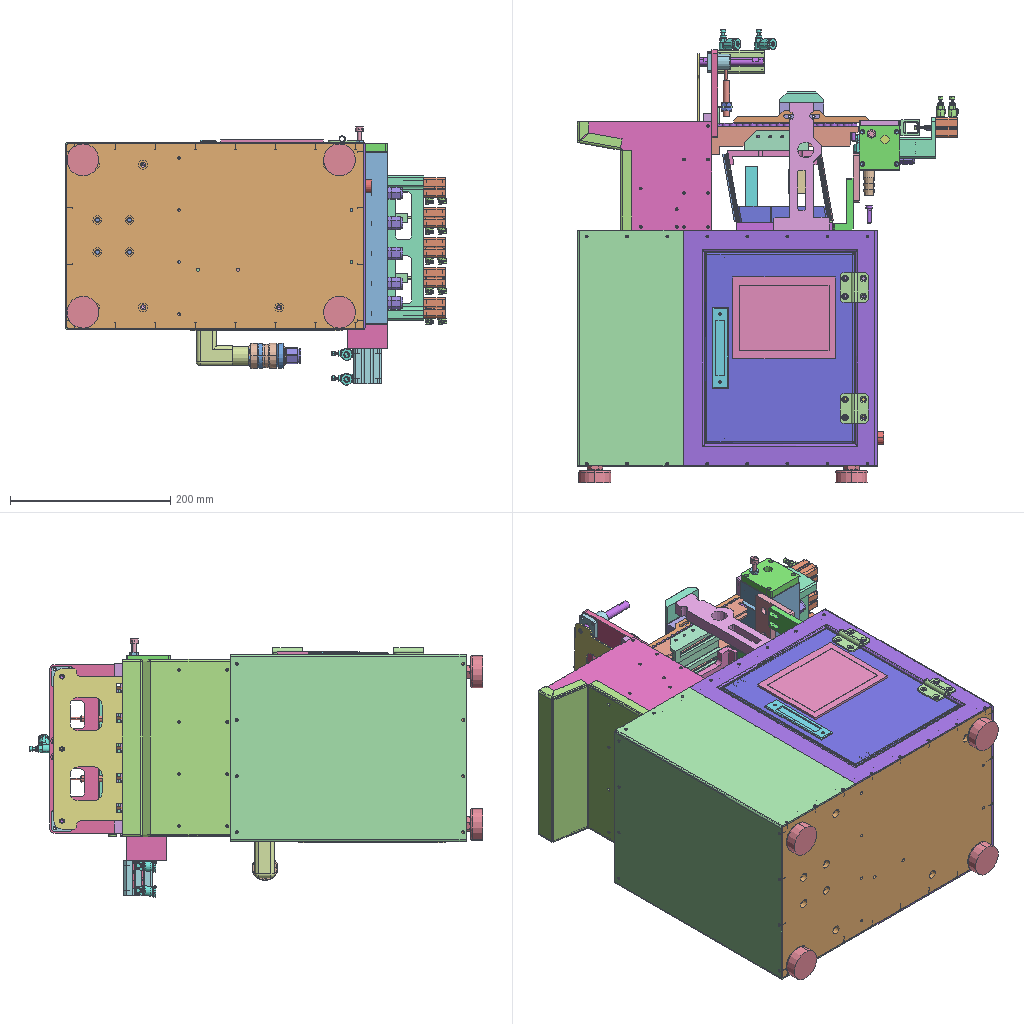Assembly | STEP file | 103 different items | 523 placed | box 476 x 566 x 322 mm
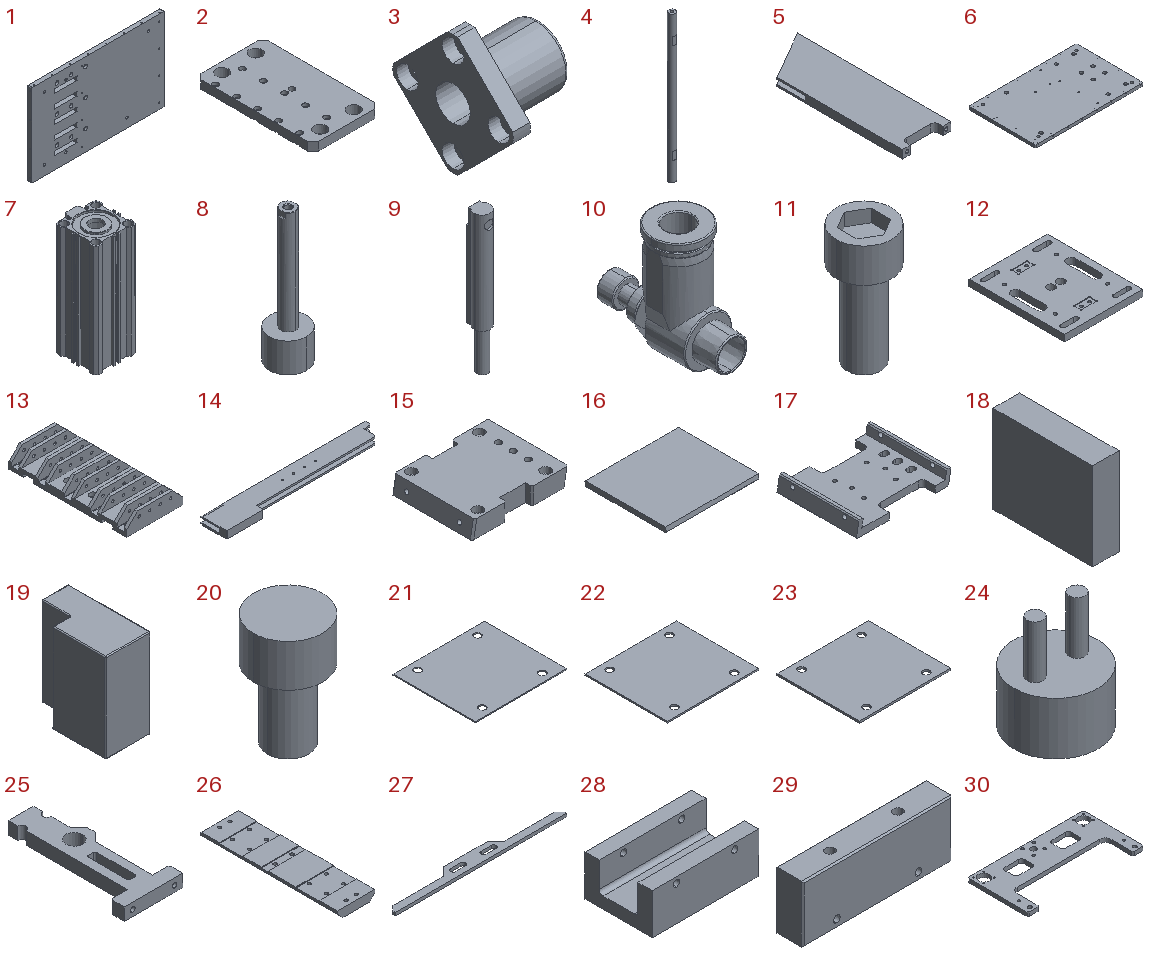Parts list (item | name | quantity | parent item | size | volume):
1 | GLSJ-10-27_default | x1 | in 202 | 370 x 12 x 230 mm | 950756 mm3
2 | GLSJ-10-31_default | x1 | in Lifting mechanism_default | 120 x 210 x 15 mm | 339737 mm3
3 | LBHSW12_default | x4 | in Lifting mechanism_default | 30 x 42 x 42 mm | 10118 mm3
4 | GLSJ-10-30_default | x6 | in Lifting mechanism_default | 12 x 12 x 272 mm | 29884 mm3
5 | GLSJ-10-32_default | x5 | in Lifting mechanism_default | 60 x 188.591 x 10 mm | 87112 mm3
6 | GLSJ-10-28_default | x1 | in Lifting mechanism_default | 370 x 230 x 10 mm | 831396 mm3
7 | HI_JSNR40X100_body_default | x1 | in JSNR40X100TD-2_07_-tab_default | 52 x 57 x 139.5 mm | 157789 mm3
8 | HI_JSNR40X100_rod_default | x1 | in JSNR40X100TD-2_07_-tab_default | 40 x 40 x 142.5 mm | 61393 mm3
9 | HI_TD-11-jsn_default | x6 | in JSNR40X100TD-2_07_-tab_default, JSNR16X30TD-2_02_-tab_default, JSNR20X15TD-2_03_-tab_default | 4 x 4.5 x 35.5 mm | 415.649 mm3
10 | KZB668-08-01-668 | x2 | in JSNR40X100TD-2_07_-tab_default | 16 x 36.5 x 33.35 mm | 5183 mm3
11 | M8 screw | x1 | in Lifting mechanism_default | 13 x 13 x 28 mm | 1901 mm3
12 | GLSJ-10-48_default | x1 | in Vibrator section_default | 120 x 147 x 10 mm | 151449 mm3
13 | GLSJ-10-12_default | x1 | in Vibrator section_default | 80 x 168 x 25 mm | 122709 mm3
14 | GLSJ-10-11_default | x5 | in Vibrator section_default | 223 x 35 x 10 mm | 29153 mm3
15 | GLSJ-10-44_default | x1 | in Vibrator_default | 113.527 x 95 x 20 mm | 189360 mm3
16 | Vibrator side plate_default | x2 | in Vibrator_default | 95 x 83.558 x 5 mm | 39344 mm3
17 | GLSJ-10-42_default | x1 | in Vibrator_default | 112.85 x 95 x 18 mm | 76999 mm3
18 | Vibrator coil left support_default | x1 | in Vibrator_default | 15 x 57 x 50 mm | 41837 mm3
19 | GLSJ-10-43_default | x1 | in Vibrator_default | 25 x 46 x 50 mm | 48561 mm3
20 | m6-15 | x5 | in Vibrator_default | 10 x 10 x 16.1 mm | 761.836 mm3
21 | GLSJ-10-45 | x10 | in Leaf spring assembly | 95 x 85 x 1 mm | 7921 mm3
22 | GLSJ-10-46 | x1 | in Vibrator_default | 95 x 85 x 1.5 mm | 11882 mm3
23 | GLSJ-10-47 | x1 | in Vibrator_default | 95 x 85 x 2 mm | 15842 mm3
24 | 332 | x1 | in Vibrator section_default | 8 x 8 x 10.1 mm | 269.13 mm3
25 | GLSJ-10-13_default | x2 | in Pressing mechanism_default | 70 x 159 x 15 mm | 69030 mm3
26 | GLSJ-10-14_default | x1 | in Pressing mechanism_default | 55 x 200 x 14 mm | 124098 mm3
27 | GLSJ-10-17_default | x5 | in Pressing mechanism_default | 170 x 15 x 3 mm | 4325 mm3
28 | GLSJ-10-15_default | x2 | in Pressing mechanism_default | 55 x 34.5 x 21 mm | 22837 mm3
29 | GLSJ-10-16_default | x1 | in Pressing mechanism_default | 55 x 10 x 21 mm | 11236 mm3
30 | GLSJ-10-21_default | x1 | in Scraper mechanism_default | 210 x 110 x 7 mm | 83543 mm3
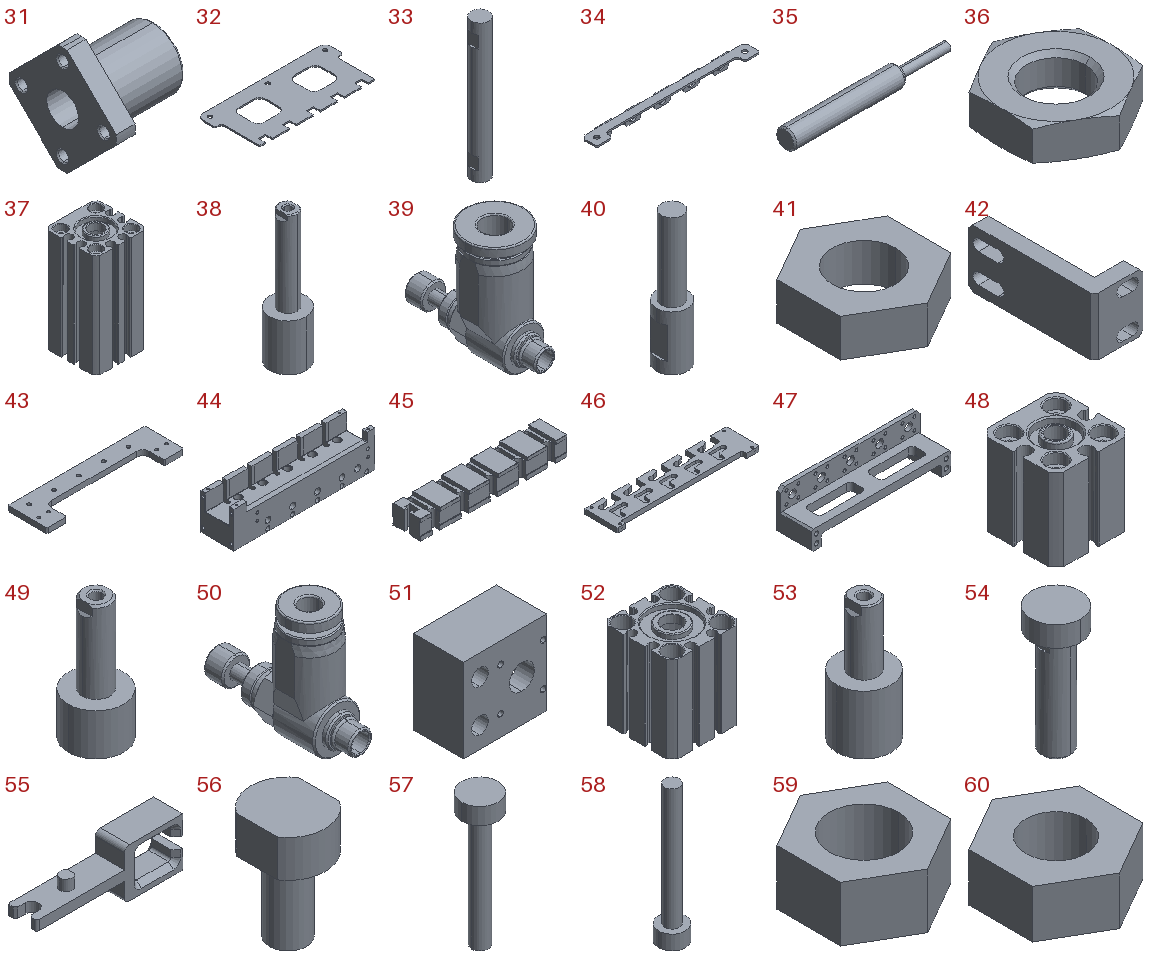31 | LHTS10_default | x2 | in Scraper mechanism_default | 29 x 34 x 34 mm | 8025 mm3
32 | GLSJ-10-18_default | x1 | in Scraper mechanism_default | 200 x 88 x 2 mm | 25026 mm3
33 | GLSJ-10-19_default | x2 | in Scraper mechanism_default | 10 x 10 x 80 mm | 5991 mm3
34 | GLSJ-10-22_default | x1 | in Scraper mechanism_default | 210 x 22.737 x 18 mm | 7535 mm3
35 | _PSAM8body_default | x5 | in PSAM8_default | 65.45 x 8 x 8 mm | 2463 mm3
36 | _PSAM8screw_default | x10 | in PSAM8_default | 13 x 15.011 x 4 mm | 426.143 mm3
37 | HI_JSNR16X30_body_default | x1 | in JSNR16X30TD-2_02_-tab_default | 29 x 29 x 58.5 mm | 29020 mm3
38 | HI_JSNR16X30_rod_default | x1 | in JSNR16X30TD-2_02_-tab_default | 16 x 16 x 58 mm | 5910 mm3
39 | KZB668-06-M5-668 | x4 | in JSNR16X30TD-2_02_-tab_default, JSNR20X15TD-2_03_-tab_default | 14 x 30.5 x 27 mm | 2988 mm3
40 | GLSJ-10-20 | x1 | in Scraper mechanism_default | 6 x 6 x 25.5 mm | 383.515 mm3
41 | M4 nut | x1 | in Scraper mechanism_default | 7 x 8.083 x 2.4 mm | 71.685 mm3
42 | GLSJ-10-01_default | x2 | in Discharge mechanism_default | 25 x 65 x 30 mm | 17211 mm3
43 | GLSJ-10-02_default | x1 | in Discharge mechanism_default | 210.5 x 60 x 8 mm | 58950 mm3
44 | GLSJ-10-03_default | x1 | in Discharge mechanism_default | 215 x 50 x 55 mm | 332871 mm3
45 | GLSJ-10-04_default | x1 | in Discharge mechanism_default | 190 x 36 x 25 mm | 119201 mm3
46 | GLSJ-10-05_default | x1 | in Discharge mechanism_default | 215 x 50 x 7 mm | 48863 mm3
47 | GLSJ-10-09_default | x1 | in Discharge mechanism_default | 180 x 45 x 51 mm | 84072 mm3
48 | HI_JSN12X10_body_default | x5 | in JSN12X10_01_-tab_default | 25 x 25 x 27 mm | 10834 mm3
49 | HI_JSN12X10_rod_default | x5 | in JSN12X10_01_-tab_default | 12 x 12 x 26.5 mm | 1467 mm3
50 | KZB668-04-M5-668 | x10 | in JSN12X10_01_-tab_default | 10.2 x 30.5 x 25.2 mm | 2441 mm3
51 | GLSJ-10-08_default | x1 | in Discharge mechanism_default | 50 x 30 x 50 mm | 46404 mm3
52 | HI_JSNR20X15_body_default | x1 | in JSNR20X15TD-2_03_-tab_default | 36 x 36 x 44.5 mm | 31416 mm3
53 | HI_JSNR20X15_rod_default | x1 | in JSNR20X15TD-2_03_-tab_default | 20 x 20 x 45 mm | 8457 mm3
54 | M5 screw_default | x299 | in Discharge mechanism_default, 202, Loose screws | 8.4 x 8.4 x 21.5 mm | 544.09 mm3
55 | Pull piece_default | x5 | in GLSJ-10-07 | 60 x 12 x 20 mm | 4860 mm3
56 | M3 screw | x5 | in GLSJ-10-07 | 5 x 6 x 9 mm | 120.482 mm3
57 | Pull rod | x1 | in Discharge mechanism_default | 11 x 11 x 40 mm | 1162 mm3
58 | M3 long screw | x5 | in Discharge mechanism_default | 5.5 x 5.5 x 28 mm | 247.989 mm3
59 | M5 nut | x2 | in Discharge mechanism_default | 8 x 9.238 x 4 mm | 143.163 mm3
60 | M3 nut | x5 | in Discharge mechanism_default | 5.5 x 6.351 x 2.4 mm | 45.909 mm3
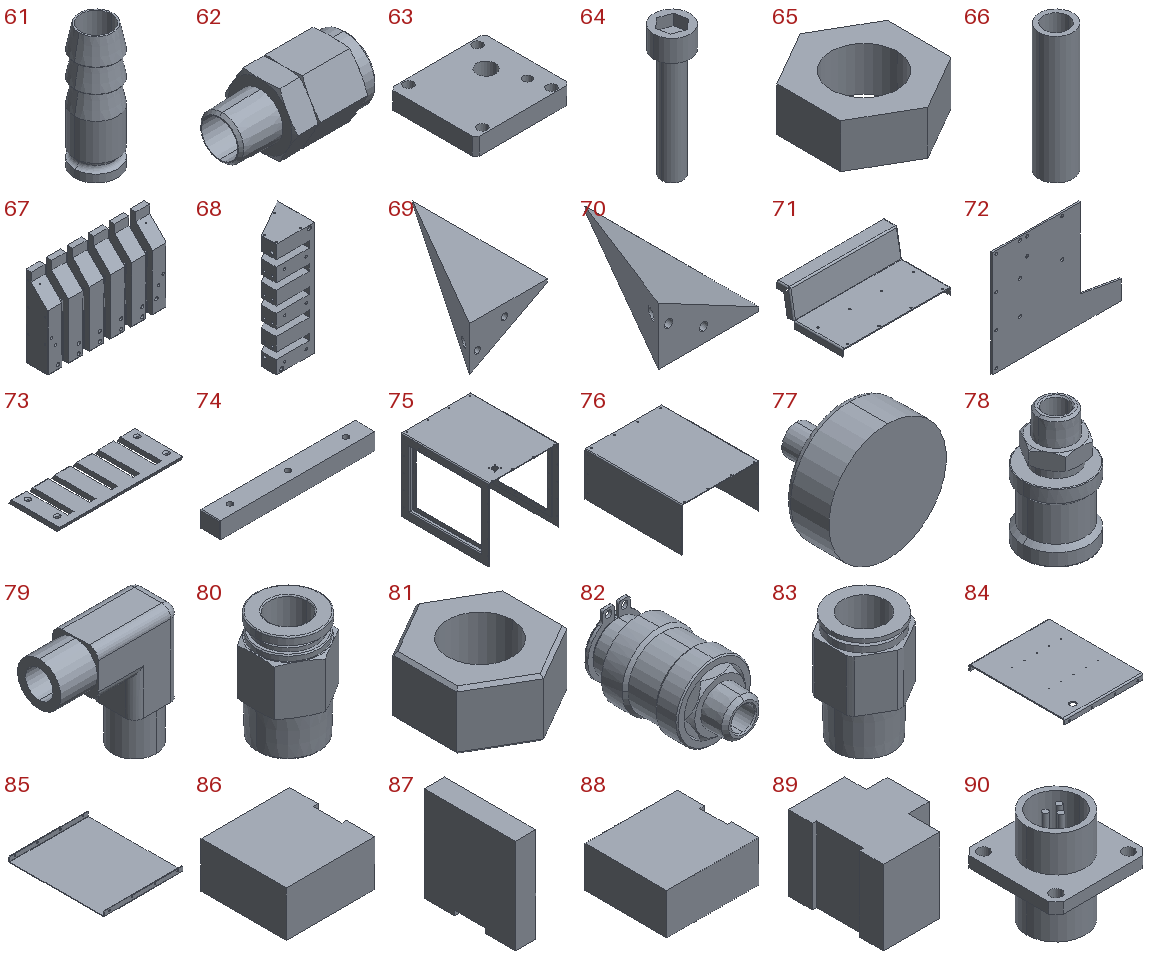61 | Air tube connector | x5 | in Discharge mechanism_default | 14 x 14 x 40 mm | 2163 mm3
62 | TJBNC8-1 | x5 | in Discharge mechanism_default | 28 x 16.166 x 14 mm | 2415 mm3
63 | GLSJ-10-06 | x1 | in Discharge mechanism_default | 55 x 50 x 10 mm | 25357 mm3
64 | M6 | x1 | in Discharge mechanism_default | 10 x 10 x 36 mm | 1220 mm3
65 | M6 nut | x1 | in Discharge mechanism_default | 10 x 11.547 x 4 mm | 233.313 mm3
66 | UM4-15 | x1 | in Discharge mechanism_default | 4 x 4 x 15 mm | 89.418 mm3
67 | GLSJ-10-24_default | x1 | in Hopper_default | 212 x 40 x 145 mm | 865440 mm3
68 | GLSJ-10-25_default | x1 | in Hopper_default | 72 x 69 x 212 mm | 565884 mm3
69 | GLSJ-10-26_default | x1 | in Hopper_default | 40.415 x 70 x 23.157 mm | 12343 mm3
70 | GLSJ-10-26(2)_default | x1 | in Hopper_default | 40.415 x 70 x 23.157 mm | 12326 mm3
71 | Screw feeder-hopper inclined plate_default | x1 | in GLSJ-10-23 | 221 x 135.003 x 67.848 mm | 86374 mm3
72 | Screw feeder-hopper side plate_default | x2 | in GLSJ-10-23 | 164 x 2 x 135 mm | 33017 mm3
73 | GLSJ-10-39 | x1 | in Hopper_default | 212 x 87.244 x 8 mm | 108665 mm3
74 | GLSJ-10-40 | x5 | in Hopper_default | 94 x 12 x 10 mm | 11056 mm3
75 | GLSJ-10-33 | x1 | in 202 | 234 x 294 x 242 mm | 310056 mm3
76 | GLSJ-10-34 | x1 | in 202 | 234 x 294 x 132 mm | 289211 mm3
77 | _pad240-10-30pad2 | x4 | in FBF40-10-30 | 40 x 31 x 40 mm | 20949 mm3
78 | VL3ME | x1 | in Air source | 31 x 31 x 58 mm | 23537 mm3
79 | GLSJ-10-35 | x1 | in Air source | 65 x 25 x 66 mm | 38293 mm3
80 | KZB175-10-03-175 | x1 | in Air source | 17 x 19.63 x 28.5 mm | 4009 mm3
81 | GLSJ-10-36 | x1 | in Air source | 36 x 41.569 x 19 mm | 14622 mm3
82 | MVHS-10A_default | x1 | in VES-10 | 31.5 x 57 x 31.5 mm | 23556 mm3
83 | GWS12-10 | x1 | in Air source | 19 x 21 x 30.5 mm | 5439 mm3
84 | GLSJ-10-38 | x1 | in 202 | 225 x 271 x 16 mm | 197957 mm3
85 | GLSJ-10-37 | x1 | in 202 | 225 x 271.5 x 14.5 mm | 99773 mm3
86 | plc | x1 | in 202 | 93.7 x 90 x 48.1 mm | 398412 mm3
87 | PLC expansion module | x1 | in 202 | 20.1 x 90 x 93.7 mm | 166488 mm3
88 | DC power supply | x1 | in 202 | 101.2 x 90.2 x 45 mm | 404021 mm3
89 | Circuit breaker | x2 | in 202 | 73 x 90 x 71 mm | 383548 mm3
90 | Aviation plug | x1 | in 202 | 26 x 26 x 26 mm | 5262 mm3
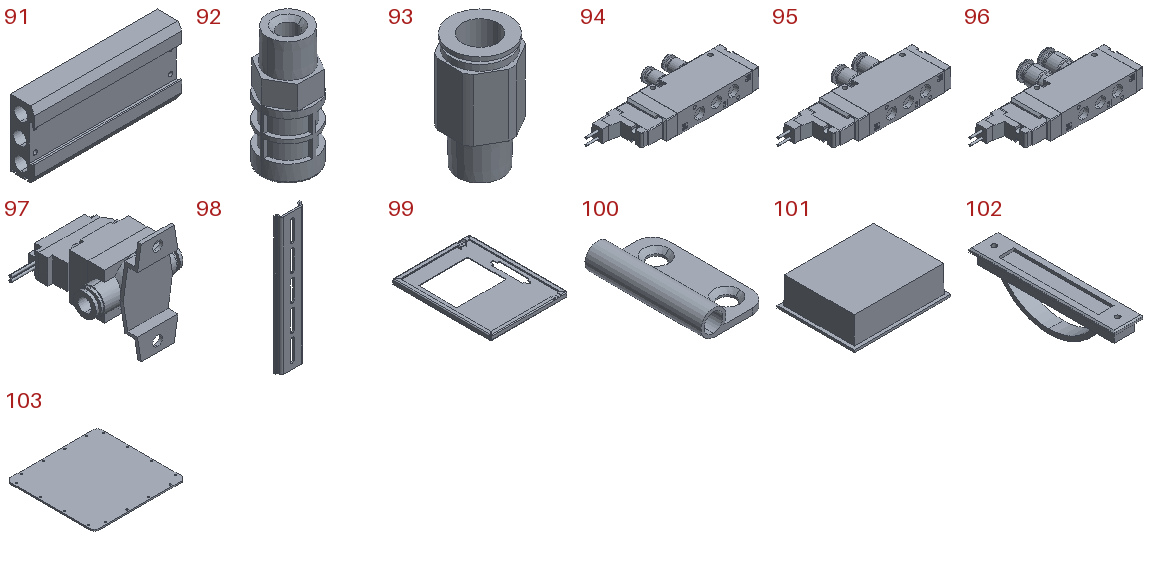91 | 8mmM4RD2-8 | x1 | in 8-station solenoid valve | 150 x 25 x 68 mm | 146651 mm3
92 | CPS1-02-S silencer | x2 | in 8-station solenoid valve | 16.166 x 16 x 36 mm | 5010 mm3
93 | GWS10-8 | x1 | in 8-station solenoid valve | 17 x 18.5 x 32.5 mm | 4848 mm3
94 | 4RD219-GS4-E2-3_default | x5 | in 44RD219-GS4-E2-3_default | 113.84 x 47.304 x 15.298 mm | 40312 mm3
95 | 4RD219-GS6-E2-3_default | x2 | in 6mm4RD219-GS6-E2-3 | 113.84 x 47.8 x 15.298 mm | 40931 mm3
96 | 4RD219-GS8-E2-3_default | x1 | in 8mm4RD219-GS8-E2-3 | 113.84 x 52.8 x 15.298 mm | 41991 mm3
97 | EXA-C8-02CB-3(1) blow-off valve | x1 | in 202 | 61.7 x 56.5 x 62 mm | 42918 mm3
98 | Guide rail | x2 | in 202 | 35 x 7.5 x 185 mm | 14405 mm3
99 | GLSJ-10-41 | x1 | in Touch screen door assembly | 186 x 238 x 12 mm | 68779 mm3
100 | heye1 | x4 | in hfl01-37 | 21.5 x 37 x 8.2 mm | 1799 mm3
101 | Touch screen | x1 | in Touch screen door assembly | 128 x 102 x 38.25 mm | 419545 mm3
102 | XAC22-100 | x1 | in Touch screen door assembly | 20 x 100 x 28.929 mm | 15353 mm3
103 | GLSJ-10-49 | x1 | in 202 | 190 x 184 x 3 mm | 104161 mm3
Placements (level | parent | child | x y z in mm | rotation matrix by rows), first 304 of 573 lines:
1 | 202 | GLSJ-10-27_default | -0.0 -0.0 -0.0 | 1 0 0 0 1 0 0 0 1
1 | 202 | Lifting mechanism_default | -233.09 -137.713 -74.013 | -1 0 0 0 0 -1 0 -1 0
2 | Lifting mechanism_default | GLSJ-10-31_default | -113.09 -74.013 -32.858 | 1 0 0 0 1 0 0 0 1
2 | Lifting mechanism_default | LBHSW12_default | -83.09 13.487 -38.858 | 0 0.7071 -0.7071 0 0.7071 0.7071 1 0 0
2 | Lifting mechanism_default | GLSJ-10-30_default | -83.09 13.487 -1.713 | 0.2532 -0.9674 0 0.9674 0.2532 0 0 0 1
2 | Lifting mechanism_default | GLSJ-10-32_default | -143.09 -149.013 -111.858 | 1 0 0 0 0 1 0 -1 -0
2 | Lifting mechanism_default | GLSJ-10-32_default | -143.09 -111.513 -111.858 | 1 0 0 0 0 1 0 -1 -0
2 | Lifting mechanism_default | GLSJ-10-32_default | -143.09 -74.013 -111.858 | 1 0 0 0 0 1 0 -1 -0
2 | Lifting mechanism_default | GLSJ-10-32_default | -143.09 -36.513 -111.858 | 1 0 0 0 0 1 0 -1 -0
2 | Lifting mechanism_default | GLSJ-10-32_default | -143.09 0.9874 -111.858 | 1 0 0 0 0 1 0 -1 -0
2 | Lifting mechanism_default | GLSJ-10-30_default | -83.09 -161.513 -1.713 | 0.5838 0.8119 0 -0.8119 0.5838 0 0 0 1
2 | Lifting mechanism_default | GLSJ-10-30_default | -143.09 -161.513 -1.713 | -0.9999 0.0173 0 -0.0173 -0.9999 0 0 0 1
2 | Lifting mechanism_default | GLSJ-10-30_default | -143.09 13.487 -1.713 | 0.4091 -0.9125 0 0.9125 0.4091 0 0 0 1
2 | Lifting mechanism_default | LBHSW12_default | -143.09 13.487 -38.858 | 0 0.7071 -0.7071 0 0.7071 0.7071 1 0 0
2 | Lifting mechanism_default | LBHSW12_default | -143.09 -161.513 -38.858 | 0 0.7071 -0.7071 0 0.7071 0.7071 1 0 0
2 | Lifting mechanism_default | LBHSW12_default | -83.09 -161.513 -38.858 | 0 0.7071 -0.7071 0 0.7071 0.7071 1 0 0
2 | Lifting mechanism_default | GLSJ-10-28_default | -233.09 -74.013 134.287 | 1 0 0 0 1 0 0 0 1
2 | Lifting mechanism_default | JSNR40X100TD-2_07_-tab_default | -106.09 -74.013 -5.213 | -1 0 0 0 1 0 0 0 -1
3 | JSNR40X100TD-2_07_-tab_default | HI_JSNR40X100_body_default | -0.0 -0.0 -0.0 | 1 0 0 0 1 0 0 0 1
3 | JSNR40X100TD-2_07_-tab_default | HI_JSNR40X100_rod_default | -0.0 0.0 5.645 | 0.9623 0.2721 0 -0.2721 0.9623 0 0 0 1
3 | JSNR40X100TD-2_07_-tab_default | HI_TD-11-jsn_default | 11.0 23.0 -0.0 | 1 0 0 0 1 0 0 0 1
3 | JSNR40X100TD-2_07_-tab_default | HI_TD-11-jsn_default | -11.0 23.0 -103.5 | 1 0 0 0 1 0 0 0 1
3 | JSNR40X100TD-2_07_-tab_default | KZB668-08-01-668 | -0.0 40.0 -11.0 | -0.6564 0 -0.7544 0 1 0 0.7544 0 -0.6564
3 | JSNR40X100TD-2_07_-tab_default | KZB668-08-01-668 | -0.0 40.0 -128.5 | 0.8837 0 0.468 0 1 0 -0.468 0 0.8837
2 | Lifting mechanism_default | M8 screw | -106.09 -74.013 -32.858 | 0.3854 -0.9227 0 -0.9227 -0.3854 0 0 0 -1
2 | Lifting mechanism_default | GLSJ-10-30_default | -373.09 -163.013 -1.713 | -0.9999 0.0173 0 -0.0173 -0.9999 0 0 0 1
2 | Lifting mechanism_default | GLSJ-10-30_default | -313.09 14.987 -1.713 | -0.9999 0.0173 0 -0.0173 -0.9999 0 0 0 1
1 | 202 | Vibrator section_default | 41.163 17.0 -17.319 | 1 0 0 0 0 1 0 -1 0
2 | Vibrator section_default | GLSJ-10-48_default | 29.837 -17.319 -5.0 | 1 0 0 0 1 0 0 0 1
2 | Vibrator section_default | GLSJ-10-12_default | 19.837 -17.319 94.739 | 1 0 0 0 1 0 0 0 1
2 | Vibrator section_default | GLSJ-10-11_default | 11.337 -92.319 107.239 | 1 0 0 0 0 -1 0 1 0
2 | Vibrator section_default | GLSJ-10-11_default | 11.337 -54.819 107.239 | 1 0 0 0 0 -1 0 1 0
2 | Vibrator section_default | GLSJ-10-11_default | 11.337 -17.319 107.239 | 1 0 0 0 0 -1 0 1 0
2 | Vibrator section_default | GLSJ-10-11_default | 11.337 20.181 107.239 | 1 0 0 0 0 -1 0 1 0
2 | Vibrator section_default | GLSJ-10-11_default | 11.337 57.681 107.239 | 1 0 0 0 0 -1 0 1 0
2 | Vibrator section_default | Vibrator_default | 38.956 -14.046 15.0 | -1 0 0 0 -1 0 0 0 1
3 | Vibrator_default | GLSJ-10-44_default | 12.568 3.274 10.0 | 1 0 0 0 1 0 0 0 1
3 | Vibrator_default | Vibrator side plate_default | -43.829 3.274 30.869 | 0 0.1736 0.9848 1 0 0 0 0.9848 -0.1736
3 | Vibrator_default | Vibrator side plate_default | 71.248 3.274 30.869 | 0 0.1736 0.9848 1 0 0 0 0.9848 -0.1736
3 | Vibrator_default | GLSJ-10-42_default | 23.455 3.274 71.739 | -1 0 0 0 1 0 0 0 -1
3 | Vibrator_default | Vibrator coil left support_default | 49.914 3.274 35.0 | 1 0 0 0 1 0 0 0 1
3 | Vibrator_default | GLSJ-10-43_default | -21.586 3.274 25.739 | -1 0 0 0 0 1 0 1 0
3 | Vibrator_default | m6-15 | -15.349 -12.726 79.739 | 1 0 0 0 1 0 0 0 1
3 | Vibrator_default | m6-15 | -15.349 3.274 79.739 | 1 0 0 0 1 0 0 0 1
3 | Vibrator_default | m6-15 | -16.786 19.274 79.739 | 0.5152 0.8571 0 -0.8571 0.5152 0 0 0 1
3 | Vibrator_default | Leaf spring assembly | 75.743 0.6075 35.454 | 0 0.1736 -0.9848 -1 0 0 0 0.9848 0.1736
4 | Leaf spring assembly | GLSJ-10-45 | -2.666 -2.537 2.631 | 1 0 0 0 1 0 0 0 1
4 | Leaf spring assembly | GLSJ-10-45 | -2.666 -2.537 1.631 | 1 0 0 0 1 0 0 0 1
4 | Leaf spring assembly | GLSJ-10-45 | -2.666 -2.537 0.6307 | 1 0 0 0 1 0 0 0 1
4 | Leaf spring assembly | GLSJ-10-45 | -2.666 -2.537 -0.3693 | 1 0 0 0 1 0 0 0 1
4 | Leaf spring assembly | GLSJ-10-45 | -2.666 -2.537 -1.369 | 1 0 0 0 1 0 0 0 1
3 | Vibrator_default | Leaf spring assembly | -39.285 0.6075 35.727 | 0 0.1736 -0.9848 -1 0 0 0 0.9848 0.1736
4 | Leaf spring assembly | GLSJ-10-45 | -2.666 -2.537 2.631 | 1 0 0 0 1 0 0 0 1
4 | Leaf spring assembly | GLSJ-10-45 | -2.666 -2.537 1.631 | 1 0 0 0 1 0 0 0 1
4 | Leaf spring assembly | GLSJ-10-45 | -2.666 -2.537 0.6307 | 1 0 0 0 1 0 0 0 1
4 | Leaf spring assembly | GLSJ-10-45 | -2.666 -2.537 -0.3693 | 1 0 0 0 1 0 0 0 1
4 | Leaf spring assembly | GLSJ-10-45 | -2.666 -2.537 -1.369 | 1 0 0 0 1 0 0 0 1
3 | Vibrator_default | m6-15 | -16.786 3.274 79.739 | 0.5152 0.8571 0 -0.8571 0.5152 0 0 0 1
3 | Vibrator_default | m6-15 | -16.786 -12.726 79.739 | 0.5152 0.8571 0 -0.8571 0.5152 0 0 0 1
3 | Vibrator_default | GLSJ-10-46 | -43.302 3.274 33.859 | 0 0.1736 -0.9848 -1 0 0 0 0.9848 0.1736
3 | Vibrator_default | GLSJ-10-47 | 76.651 3.274 32.717 | 0 0.1736 0.9848 1 0 0 0 0.9848 -0.1736
2 | Vibrator section_default | 332 | -93.34 -92.319 129.739 | -1 0 0 0 1 0 0 0 -1
1 | 202 | Pressing mechanism_default | 51.966 83.662 92.5 | 1 0 0 0 1 0 0 0 1
2 | Pressing mechanism_default | GLSJ-10-13_default | 41.034 -55.662 -0.0 | 1 0 0 0 1 0 0 0 1
2 | Pressing mechanism_default | GLSJ-10-14_default | 41.034 101.338 -92.5 | 1 0 0 0 0 -1 0 1 0
2 | Pressing mechanism_default | GLSJ-10-13_default | 41.034 -55.662 -185.0 | 1 0 0 0 1 0 0 0 1
2 | Pressing mechanism_default | GLSJ-10-17_default | 41.034 70.338 -16.0 | -1 0 0 0 1 0 0 0 -1
2 | Pressing mechanism_default | GLSJ-10-17_default | 41.034 70.338 -53.5 | -1 0 0 0 1 0 0 0 -1
2 | Pressing mechanism_default | GLSJ-10-17_default | 41.034 70.338 -91.0 | -1 0 0 0 1 0 0 0 -1
2 | Pressing mechanism_default | GLSJ-10-17_default | 41.034 70.338 -128.5 | -1 0 0 0 1 0 0 0 -1
2 | Pressing mechanism_default | GLSJ-10-17_default | 41.034 70.338 -166.0 | -1 0 0 0 1 0 0 0 -1
2 | Pressing mechanism_default | GLSJ-10-15_default | 41.034 100.838 -205.0 | 1 0 0 0 0 -1 0 1 -0
2 | Pressing mechanism_default | GLSJ-10-16_default | 41.034 67.338 -86.0 | 1 0 0 0 0 1 0 -1 0
2 | Pressing mechanism_default | GLSJ-10-15_default | 41.034 100.838 -92.5 | 1 0 0 0 0 -1 0 1 -0
1 | 202 | Scraper mechanism_default | -19.0 172.997 -22.279 | 0 0 1 0 1 0 -1 0 0
2 | Scraper mechanism_default | GLSJ-10-21_default | -21.279 9.003 0.0 | 1 0 0 0 1 0 0 0 1
2 | Scraper mechanism_default | LHTS10_default | -111.279 49.003 -6.0 | 0 0.7071 -0.7071 0 0.7071 0.7071 1 0 0
2 | Scraper mechanism_default | LHTS10_default | 68.721 49.003 -6.0 | 0 0.7071 -0.7071 0 0.7071 0.7071 1 0 0
2 | Scraper mechanism_default | GLSJ-10-18_default | -21.279 15.003 -18.0 | 1 0 0 0 1 0 0 0 1
2 | Scraper mechanism_default | GLSJ-10-19_default | 68.721 49.003 -16.0 | -0.9145 0.4045 0 -0.4045 -0.9145 0 0 0 1
2 | Scraper mechanism_default | GLSJ-10-19_default | -111.279 49.003 -16.0 | -0.7793 -0.6267 0 0.6267 -0.7793 0 0 0 1
2 | Scraper mechanism_default | GLSJ-10-22_default | -21.279 -18.997 7.0 | -1 0 0 0 1 0 0 0 -1
2 | Scraper mechanism_default | PSAM8_default | -95.992 -19.379 18.233 | 0 -1 0 1 0 0 0 0 1
3 | PSAM8_default | _PSAM8body_default | 0.1184 0.2874 -0.2326 | 1 0 0 0 1 0 0 0 1
3 | PSAM8_default | _PSAM8screw_default | 11.118 0.2874 -0.2326 | 0 0 -1 0 -1 0 -1 0 0
3 | PSAM8_default | _PSAM8screw_default | 17.118 0.2874 -0.2326 | 0 0 -1 0 -1 0 -1 0 0
2 | Scraper mechanism_default | PSAM8_default | -58.492 -19.379 18.233 | 0 -1 0 1 0 0 0 0 1
3 | PSAM8_default | _PSAM8body_default | 0.1184 0.2874 -0.2326 | 1 0 0 0 1 0 0 0 1
3 | PSAM8_default | _PSAM8screw_default | 11.118 0.2874 -0.2326 | 0 0 -1 0 -1 0 -1 0 0
3 | PSAM8_default | _PSAM8screw_default | 17.118 0.2874 -0.2326 | 0 0 -1 0 -1 0 -1 0 0
2 | Scraper mechanism_default | PSAM8_default | -20.992 -19.379 18.233 | 0 -1 0 1 0 0 0 0 1
3 | PSAM8_default | _PSAM8body_default | 0.1184 0.2874 -0.2326 | 1 0 0 0 1 0 0 0 1
3 | PSAM8_default | _PSAM8screw_default | 11.118 0.2874 -0.2326 | 0 0 -1 0 -1 0 -1 0 0
3 | PSAM8_default | _PSAM8screw_default | 17.118 0.2874 -0.2326 | 0 0 -1 0 -1 0 -1 0 0
2 | Scraper mechanism_default | PSAM8_default | 16.508 -19.379 18.233 | 0 -1 0 1 0 0 0 0 1
3 | PSAM8_default | _PSAM8body_default | 0.1184 0.2874 -0.2326 | 1 0 0 0 1 0 0 0 1
3 | PSAM8_default | _PSAM8screw_default | 11.118 0.2874 -0.2326 | 0 0 -1 0 -1 0 -1 0 0
3 | PSAM8_default | _PSAM8screw_default | 17.118 0.2874 -0.2326 | 0 0 -1 0 -1 0 -1 0 0
2 | Scraper mechanism_default | PSAM8_default | 54.008 -19.379 18.233 | 0 -1 0 1 0 0 0 0 1
3 | PSAM8_default | _PSAM8body_default | 0.1184 0.2874 -0.2326 | 1 0 0 0 1 0 0 0 1
3 | PSAM8_default | _PSAM8screw_default | 11.118 0.2874 -0.2326 | 0 0 -1 0 -1 0 -1 0 0
3 | PSAM8_default | _PSAM8screw_default | 17.118 0.2874 -0.2326 | 0 0 -1 0 -1 0 -1 0 0
2 | Scraper mechanism_default | JSNR16X30TD-2_02_-tab_default | -21.279 49.003 7.0 | -1 0 0 0 1 0 0 0 -1
3 | JSNR16X30TD-2_02_-tab_default | HI_JSNR16X30_body_default | -0.0 0.0 0.0 | 1 0 0 0 1 0 0 0 1
3 | JSNR16X30TD-2_02_-tab_default | HI_JSNR16X30_rod_default | -0.0 -0.0 0.0 | 0.7351 0.678 0 -0.678 0.7351 0 0 0 1
3 | JSNR16X30TD-2_02_-tab_default | HI_TD-11-jsn_default | 11.6 3.5 0.0 | 0 1 0 -1 0 0 0 0 1
3 | JSNR16X30TD-2_02_-tab_default | HI_TD-11-jsn_default | 11.6 -3.5 -22.5 | 0 1 0 -1 0 0 0 0 1
3 | JSNR16X30TD-2_02_-tab_default | KZB668-06-M5-668 | -0.0 22.5 -51.5 | -0.8067 0 0.5909 0 1 0 -0.5909 0 -0.8067
3 | JSNR16X30TD-2_02_-tab_default | KZB668-06-M5-668 | -0.0 22.5 -7.0 | -0.8239 0 0.5668 0 1 0 -0.5668 0 -0.8239
2 | Scraper mechanism_default | GLSJ-10-20 | -21.279 49.003 -16.0 | -0.2416 -0.9704 0 0.9704 -0.2416 0 0 0 1
2 | Scraper mechanism_default | M4 nut | -21.279 49.003 1.1 | 1 0 0 0 1 0 0 0 1
1 | 202 | Discharge mechanism_default | 144.058 43.876 -90.25 | -1 0 0 0 1 0 0 0 -1
2 | Discharge mechanism_default | GLSJ-10-01_default | -12.942 -31.876 -0.0 | 1 0 0 0 1 0 0 0 1
2 | Discharge mechanism_default | GLSJ-10-02_default | -12.942 33.124 -90.25 | 0 0 -1 0 1 0 1 0 -0
2 | Discharge mechanism_default | GLSJ-10-03_default | -45.942 43.124 -88.0 | 0 1 0 0 0 1 1 0 -0
2 | Discharge mechanism_default | GLSJ-10-04_default | -45.942 73.124 -75.5 | 0 -1 0 0 0 1 -1 0 -0
2 | Discharge mechanism_default | GLSJ-10-01_default | -12.942 -31.876 -180.5 | 1 0 0 0 1 0 0 0 1
2 | Discharge mechanism_default | GLSJ-10-05_default | -45.942 105.124 -88.0 | 0 1 0 0 0 -1 -1 0 -0
2 | Discharge mechanism_default | GLSJ-10-09_default | -90.942 58.124 -75.5 | 0 -1 0 0 0 1 -1 0 -0
2 | Discharge mechanism_default | JSN12X10_01_-tab_default | -117.505 95.021 -153.166 | 0 0 1 0 1 0 -1 0 -0
3 | JSN12X10_01_-tab_default | HI_JSN12X10_body_default | -2.666 1.103 1.563 | 1 0 0 0 1 0 0 0 1
3 | JSN12X10_01_-tab_default | HI_JSN12X10_rod_default | -2.666 1.103 1.563 | -0.9031 -0.4294 0 0.4294 -0.9031 0 0 0 1
3 | JSN12X10_01_-tab_default | KZB668-04-M5-668 | -2.666 20.603 -19.237 | -0.153 0 -0.9882 0 1 0 0.9882 0 -0.153
3 | JSN12X10_01_-tab_default | KZB668-04-M5-668 | -2.666 20.603 -4.637 | -0.06201 0 -0.9981 0 1 0 0.9981 0 -0.06201
2 | Discharge mechanism_default | JSN12X10_01_-tab_default | -117.505 95.021 -115.665 | 0 0 1 0 1 0 -1 0 -0
3 | JSN12X10_01_-tab_default | HI_JSN12X10_body_default | -2.666 1.103 1.563 | 1 0 0 0 1 0 0 0 1
3 | JSN12X10_01_-tab_default | HI_JSN12X10_rod_default | -2.666 1.103 1.563 | -0.9031 -0.4294 0 0.4294 -0.9031 0 0 0 1
3 | JSN12X10_01_-tab_default | KZB668-04-M5-668 | -2.666 20.603 -19.237 | -0.153 0 -0.9882 0 1 0 0.9882 0 -0.153
3 | JSN12X10_01_-tab_default | KZB668-04-M5-668 | -2.666 20.603 -4.637 | -0.06201 0 -0.9981 0 1 0 0.9981 0 -0.06201
2 | Discharge mechanism_default | JSN12X10_01_-tab_default | -117.505 95.021 -78.165 | 0 0 1 0 1 0 -1 0 -0
3 | JSN12X10_01_-tab_default | HI_JSN12X10_body_default | -2.666 1.103 1.563 | 1 0 0 0 1 0 0 0 1
3 | JSN12X10_01_-tab_default | HI_JSN12X10_rod_default | -2.666 1.103 1.563 | -0.9031 -0.4294 0 0.4294 -0.9031 0 0 0 1
3 | JSN12X10_01_-tab_default | KZB668-04-M5-668 | -2.666 20.603 -19.237 | -0.153 0 -0.9882 0 1 0 0.9882 0 -0.153
3 | JSN12X10_01_-tab_default | KZB668-04-M5-668 | -2.666 20.603 -4.637 | -0.06201 0 -0.9981 0 1 0 0.9981 0 -0.06201
2 | Discharge mechanism_default | JSN12X10_01_-tab_default | -117.505 95.021 -40.666 | 0 0 1 0 1 0 -1 0 -0
3 | JSN12X10_01_-tab_default | HI_JSN12X10_body_default | -2.666 1.103 1.563 | 1 0 0 0 1 0 0 0 1
3 | JSN12X10_01_-tab_default | HI_JSN12X10_rod_default | -2.666 1.103 1.563 | -0.9031 -0.4294 0 0.4294 -0.9031 0 0 0 1
3 | JSN12X10_01_-tab_default | KZB668-04-M5-668 | -2.666 20.603 -19.237 | -0.153 0 -0.9882 0 1 0 0.9882 0 -0.153
3 | JSN12X10_01_-tab_default | KZB668-04-M5-668 | -2.666 20.603 -4.637 | -0.06201 0 -0.9981 0 1 0 0.9981 0 -0.06201
2 | Discharge mechanism_default | JSN12X10_01_-tab_default | -117.505 95.021 -3.166 | 0 0 1 0 1 0 -1 0 -0
3 | JSN12X10_01_-tab_default | HI_JSN12X10_body_default | -2.666 1.103 1.563 | 1 0 0 0 1 0 0 0 1
3 | JSN12X10_01_-tab_default | HI_JSN12X10_rod_default | -2.666 1.103 11.563 | -0.1241 0.9923 0 -0.9923 -0.1241 0 0 0 1
3 | JSN12X10_01_-tab_default | KZB668-04-M5-668 | -2.666 20.603 -19.237 | -0.153 0 -0.9882 0 1 0 0.9882 0 -0.153
3 | JSN12X10_01_-tab_default | KZB668-04-M5-668 | -2.666 20.603 -4.637 | -0.06201 0 -0.9981 0 1 0 0.9981 0 -0.06201
2 | Discharge mechanism_default | GLSJ-10-08_default | -45.942 73.124 49.5 | 0 0 -1 1 0 0 0 -1 0
2 | Discharge mechanism_default | JSNR20X15TD-2_03_-tab_default | -45.942 83.124 49.5 | 0 1 0 1 0 0 0 0 -1
3 | JSNR20X15TD-2_03_-tab_default | HI_JSNR20X15_body_default | 0.0 -0.0 -0.0 | 1 0 0 0 1 0 0 0 1
3 | JSNR20X15TD-2_03_-tab_default | HI_JSNR20X15_rod_default | 0.0 -0.0 -0.0 | 0.9823 0.1871 0 -0.1871 0.9823 0 0 0 1
3 | JSNR20X15TD-2_03_-tab_default | HI_TD-11-jsn_default | 5.5 14.9 -0.0 | 1 0 0 0 1 0 0 0 1
3 | JSNR20X15TD-2_03_-tab_default | HI_TD-11-jsn_default | -5.5 14.9 -8.5 | 1 0 0 0 1 0 0 0 1
3 | JSNR20X15TD-2_03_-tab_default | KZB668-06-M5-668 | -0.0 26.0 -37.7 | -0.07357 0 -0.9973 0 1 0 0.9973 0 -0.07357
3 | JSNR20X15TD-2_03_-tab_default | KZB668-06-M5-668 | 0.0 26.0 -6.8 | -0.07357 0 -0.9973 0 1 0 0.9973 0 -0.07357
2 | Discharge mechanism_default | M5 screw_default | -32.942 83.124 -0.5 | 0.9788 -0.2048 0 0 0 1 -0.2048 -0.9788 -0
2 | Discharge mechanism_default | M5 screw_default | -32.942 83.124 -38.0 | 0.9788 -0.2048 0 0 0 1 -0.2048 -0.9788 -0
2 | Discharge mechanism_default | M5 screw_default | -32.942 83.124 -75.5 | 0.9788 -0.2048 0 0 0 1 -0.2048 -0.9788 -0
2 | Discharge mechanism_default | M5 screw_default | -32.942 83.124 -150.5 | 0.8634 -0.5045 0 0 0 1 -0.5045 -0.8634 0
2 | Discharge mechanism_default | M5 screw_default | -32.942 83.124 -113.0 | 0.9788 -0.2048 0 0 0 1 -0.2048 -0.9788 0
2 | Discharge mechanism_default | GLSJ-10-07 | -75.593 103.181 -3.391 | -1 0 0 0 0 -1 0 -1 0
3 | GLSJ-10-07 | Pull piece_default | -9.651 -2.891 7.057 | 1 0 0 0 1 0 0 0 1
3 | GLSJ-10-07 | M3 screw | -21.651 -2.891 5.057 | 1 0 0 0 -1 0 0 0 -1
2 | Discharge mechanism_default | GLSJ-10-07 | -75.593 103.181 -40.891 | -1 0 0 0 0 -1 0 -1 0
3 | GLSJ-10-07 | Pull piece_default | -9.651 -2.891 7.057 | 1 0 0 0 1 0 0 0 1
3 | GLSJ-10-07 | M3 screw | -21.651 -2.891 5.057 | 1 0 0 0 -1 0 0 0 -1
2 | Discharge mechanism_default | GLSJ-10-07 | -75.593 103.181 -78.391 | -1 0 0 0 0 -1 0 -1 0
3 | GLSJ-10-07 | Pull piece_default | -9.651 -2.891 7.057 | 1 0 0 0 1 0 0 0 1
3 | GLSJ-10-07 | M3 screw | -21.651 -2.891 5.057 | 1 0 0 0 -1 0 0 0 -1
2 | Discharge mechanism_default | GLSJ-10-07 | -75.593 103.181 -115.891 | -1 0 0 0 0 -1 0 -1 0
3 | GLSJ-10-07 | Pull piece_default | -9.651 -2.891 7.057 | 1 0 0 0 1 0 0 0 1
3 | GLSJ-10-07 | M3 screw | -21.651 -2.891 5.057 | 1 0 0 0 -1 0 0 0 -1
2 | Discharge mechanism_default | GLSJ-10-07 | -75.593 103.181 -153.391 | -1 0 0 0 0 -1 0 -1 0
3 | GLSJ-10-07 | Pull piece_default | -9.651 -2.891 7.057 | 1 0 0 0 1 0 0 0 1
3 | GLSJ-10-07 | M3 screw | -21.651 -2.891 5.057 | 1 0 0 0 -1 0 0 0 -1
2 | Discharge mechanism_default | Pull rod | -45.942 83.124 15.5 | -0.213 -0.9771 0 -0.9771 0.213 0 0 0 -1
2 | Discharge mechanism_default | M3 long screw | -89.442 96.124 -0.5 | 0 0 -1 -0.9397 -0.342 0 -0.342 0.9397 0
2 | Discharge mechanism_default | M5 nut | -45.942 83.124 41.0 | 1 0 0 0 1 0 0 0 1
2 | Discharge mechanism_default | M5 nut | -45.942 83.124 19.5 | 1 0 0 0 1 0 0 0 1
2 | Discharge mechanism_default | M3 nut | -110.042 96.124 -0.5 | 0 0 -1 0.902 0.4317 0 0.4317 -0.902 -0
2 | Discharge mechanism_default | M3 long screw | -89.442 96.124 -75.5 | 0 0 -1 0.9428 -0.3335 0 -0.3335 -0.9428 0
2 | Discharge mechanism_default | M3 long screw | -89.442 96.124 -38.0 | 0 0 -1 0.9428 -0.3335 0 -0.3335 -0.9428 0
2 | Discharge mechanism_default | M3 long screw | -89.442 96.124 -150.5 | 0 0 -1 0.3807 -0.9247 0 -0.9247 -0.3807 0
2 | Discharge mechanism_default | M3 long screw | -89.442 96.124 -113.0 | 0 0 -1 0.9428 -0.3335 0 -0.3335 -0.9428 0
2 | Discharge mechanism_default | M3 nut | -110.042 96.124 -38.0 | 0 0 -1 0.902 0.4317 0 0.4317 -0.902 -0
2 | Discharge mechanism_default | M3 nut | -110.042 96.124 -150.5 | 0 0 -1 0.902 0.4317 0 0.4317 -0.902 -0
2 | Discharge mechanism_default | M3 nut | -110.042 96.124 -113.0 | 0 0 -1 0.902 0.4317 0 0.4317 -0.902 -0
2 | Discharge mechanism_default | M3 nut | -110.042 96.124 -75.5 | 0 0 -1 0.902 0.4317 0 0.4317 -0.902 -0
2 | Discharge mechanism_default | M5 screw_default | -42.6 83.124 -150.5 | 0 -1 0 0 0 1 -1 0 0
2 | Discharge mechanism_default | Air tube connector | -32.942 51.124 -0.5 | 0.9015 -0.4328 0 0 0 -1 0.4328 0.9015 0
2 | Discharge mechanism_default | Air tube connector | -32.942 51.124 -38.0 | 0.9015 -0.4328 0 0 0 -1 0.4328 0.9015 0
2 | Discharge mechanism_default | Air tube connector | -32.942 51.124 -150.5 | 0.9015 -0.4328 0 0 0 -1 0.4328 0.9015 0
2 | Discharge mechanism_default | Air tube connector | -32.942 51.124 -75.5 | 0.9015 -0.4328 0 0 0 -1 0.4328 0.9015 0
2 | Discharge mechanism_default | Air tube connector | -32.942 51.124 -113.0 | 0.9015 -0.4328 0 0 0 -1 0.4328 0.9015 0
2 | Discharge mechanism_default | TJBNC8-1 | -70.942 58.124 -7.25 | -1 0 0 0 0.9211 0.3894 0 0.3894 -0.9211
2 | Discharge mechanism_default | TJBNC8-1 | -70.942 58.124 -31.0 | -1 0 0 0 0.9211 0.3894 0 0.3894 -0.9211
2 | Discharge mechanism_default | TJBNC8-1 | -70.942 58.124 -68.5 | -1 0 0 0 0.9211 0.3894 0 0.3894 -0.9211
2 | Discharge mechanism_default | TJBNC8-1 | -70.942 58.124 -106.0 | -1 0 0 0 0.9211 0.3894 0 0.3894 -0.9211
2 | Discharge mechanism_default | TJBNC8-1 | -70.942 58.124 -143.5 | -1 0 0 0 -0.6234 0.7819 0 0.7819 0.6234
2 | Discharge mechanism_default | GLSJ-10-06 | -45.942 70.624 -205.5 | 0 -1 0 1 0 0 0 0 1
2 | Discharge mechanism_default | M6 | -35.942 88.124 -220.5 | -0.8632 -0.5048 0 -0.5048 0.8632 0 0 0 -1
2 | Discharge mechanism_default | M6 nut | -35.942 88.124 -209.5 | 1 0 0 0 1 0 0 0 1
2 | Discharge mechanism_default | UM4-15 | -55.042 96.224 -15.25 | 0 0 -1 -0.4423 0.8969 0 0.8969 0.4423 -0
2 | Discharge mechanism_default | M5 screw_default | -32.942 -19.818 -150.5 | -0.7211 -0.6928 0 0 0 1 -0.6928 0.7211 0
2 | Discharge mechanism_default | M5 screw_default | -32.942 -19.818 -0.5 | -0.288 -0.9576 0 0 0 1 -0.9576 0.288 0
1 | 202 | Hopper_default | -28.36 92.0 -20.952 | 0 1 0 0 0 1 1 0 0
2 | Hopper_default | GLSJ-10-24_default | 20.952 -10.639 -80.0 | 1 0 0 0 1 0 0 0 1
2 | Hopper_default | GLSJ-10-25_default | 20.952 -66.639 -45.5 | 0 0 -1 -1 0 0 0 1 -0
2 | Hopper_default | GLSJ-10-26_default | 102.952 -30.64 -2.628 | 0 0 1 0 -1 0 1 0 -0
2 | Hopper_default | GLSJ-10-26(2)_default | -61.048 -30.64 -2.628 | 0 0 1 0 -1 0 1 0 0
2 | Hopper_default | GLSJ-10-23 | 60.81 -110.504 -22.679 | 1 0 0 0 0 -1 0 1 -0
3 | GLSJ-10-23 | Screw feeder-hopper inclined plate_default | -39.859 -7.321 -5.865 | 1 0 0 0 1 0 0 0 1
3 | GLSJ-10-23 | Screw feeder-hopper side plate_default | 66.641 10.179 -63.865 | 0 -1 0 0 0 -1 1 0 0
3 | GLSJ-10-23 | Screw feeder-hopper side plate_default | -148.359 10.179 -63.865 | 0 -1 0 0 0 -1 1 0 0
2 | Hopper_default | GLSJ-10-39 | 20.952 -66.58 -31.53 | 1 0 0 0 0.866 0.5 0 -0.5 0.866
2 | Hopper_default | GLSJ-10-40 | -54.048 -30.64 -33.0 | 0 -1 0 0 0 1 -1 0 0
2 | Hopper_default | GLSJ-10-40 | -16.548 -30.64 -33.0 | 0 -1 0 0 0 1 -1 0 0
2 | Hopper_default | GLSJ-10-40 | 20.952 -30.64 -33.0 | 0 -1 0 0 0 1 -1 0 0
2 | Hopper_default | GLSJ-10-40 | 58.452 -30.64 -33.0 | 0 -1 0 0 0 1 -1 0 0
2 | Hopper_default | GLSJ-10-40 | 95.952 -30.64 -33.0 | 0 -1 0 0 0 1 -1 0 0
1 | 202 | M5 screw_default | -81.782 43.4 75.0 | 0 -0.866 0.5 0 0.5 0.866 -1 0 0
1 | 202 | M5 screw_default | 152.222 126.739 75.0 | 0 -1 0 0 0 1 -1 0 0
1 | 202 | M5 screw_default | -52.377 126.739 75.0 | 0 -1 0 0 0 1 -1 0 0
1 | 202 | GLSJ-10-33 | 187.0 -135.0 -0.0 | 0 0 1 0 1 0 -1 0 0
1 | 202 | GLSJ-10-34 | -187.0 -135.0 0.0 | 0 0 -1 0 1 0 1 0 0
1 | 202 | FBF40-10-30 | 155.0 -299.894 -95.0 | 1 0 0 0 1 0 0 0 1
2 | FBF40-10-30 | _pad240-10-30pad2 | -0.0 -3.106 -0.0 | 1 0 0 0 1 0 0 0 1
1 | 202 | FBF40-10-30 | 155.0 -299.894 95.0 | 1 0 0 0 1 0 0 0 1
2 | FBF40-10-30 | _pad240-10-30pad2 | -0.0 -3.106 -0.0 | 1 0 0 0 1 0 0 0 1
1 | 202 | FBF40-10-30 | -165.0 -299.894 -95.0 | 0.9608 0 0.2774 0 1 0 -0.2774 0 0.9608
2 | FBF40-10-30 | _pad240-10-30pad2 | -0.0 -3.106 -0.0 | 1 0 0 0 1 0 0 0 1
1 | 202 | FBF40-10-30 | -165.0 -299.894 95.0 | 1 0 0 0 1 0 0 0 1
2 | FBF40-10-30 | _pad240-10-30pad2 | -0.0 -3.106 -0.0 | 1 0 0 0 1 0 0 0 1
1 | 202 | Air source | 67.298 -28.211 -137.467 | 0 0 -1 0 1 0 1 0 -0
2 | Air source | VL3ME | -12.033 -2.789 37.298 | 1 0 0 0 1 0 0 0 1
2 | Air source | GLSJ-10-35 | -12.033 -2.789 45.798 | 0 0 -1 0 1 0 1 0 -0
2 | Air source | KZB175-10-03-175 | 31.467 -2.789 78.298 | 0 0 1 0.6546 0.756 0 -0.756 0.6546 0
2 | Air source | GLSJ-10-36 | 22.467 -2.789 78.298 | 0 0 1 -0.1793 0.9838 0 -0.9838 -0.1793 0
2 | Air source | VES-10 | -12.033 -2.789 23.298 | -1 0 -0.00404 0.00404 0 -1 0 -1 0
3 | VES-10 | MVHS-10A_default | 0.0 16.0 -0.0 | 1 0 0 0 1 0 0 0 1
2 | Air source | GWS12-10 | -12.033 -2.789 -39.702 | 0.6089 -0.7933 0 -0.7933 -0.6089 0 0 0 -1
1 | 202 | GLSJ-10-38 | 181.0 -136.5 0.0 | 0 0 1 0 1 0 -1 0 0
1 | 202 | GLSJ-10-37 | -53.5 -136.25 0.0 | 0 0 1 0 1 0 -1 0 0
1 | 202 | plc | 128.65 -176.5 -13.6 | 1 0 0 0 1 0 0 0 1
1 | 202 | PLC expansion module | 175.5 -176.5 56.55 | 0 0 -1 0 1 0 1 0 -0
1 | 202 | DC power supply | 124.9 -71.5 -10.5 | 1 0 0 0 1 0 0 0 1
1 | 202 | Circuit breaker | 138.0 -71.5 -20.5 | -1 0 0 0 1 0 0 0 -1
1 | 202 | Aviation plug | 182.0 -247.0 62.5 | 0 0 1 0 1 0 -1 0 0
1 | 202 | Circuit breaker | 138.0 -176.5 -20.5 | -1 0 0 0 1 0 0 0 -1
1 | 202 | 8-station solenoid valve | -46.507 -132.324 -48.5 | 0 1 0 1 0 0 0 0 -1
2 | 8-station solenoid valve | 8mmM4RD2-8 | -181.274 18.007 -0.2 | 1 0 0 0 1 0 0 0 1
2 | 8-station solenoid valve | CPS1-02-S silencer | 87.226 7.007 -22.0 | 0 0 -1 0.2078 0.9782 0 0.9782 -0.2078 0
2 | 8-station solenoid valve | CPS1-02-S silencer | 87.226 7.007 22.0 | 0 0 -1 -0.3505 0.9366 0 0.9366 0.3505 0
2 | 8-station solenoid valve | GWS10-8 | 92.226 8.007 -0.0 | 0 0 1 1 -0.00298 0 0.00298 1 -0
2 | 8-station solenoid valve | 44RD219-GS4-E2-3_default | -60.825 31.507 -28.8 | 0 0 -1 0 1 0 1 0 -0
3 | 44RD219-GS4-E2-3_default | 4RD219-GS4-E2-3_default | 0.0 0.0 -0.0 | 1 0 0 0 1 0 0 0 1
2 | 8-station solenoid valve | 44RD219-GS4-E2-3_default | -44.825 31.507 -28.8 | 0 0 -1 0 1 0 1 0 -0
3 | 44RD219-GS4-E2-3_default | 4RD219-GS4-E2-3_default | 0.0 0.0 -0.0 | 1 0 0 0 1 0 0 0 1
2 | 8-station solenoid valve | 44RD219-GS4-E2-3_default | -28.825 31.507 -28.8 | 0 0 -1 0 1 0 1 0 -0
3 | 44RD219-GS4-E2-3_default | 4RD219-GS4-E2-3_default | 0.0 0.0 -0.0 | 1 0 0 0 1 0 0 0 1
2 | 8-station solenoid valve | 44RD219-GS4-E2-3_default | -12.825 31.507 -28.8 | 0 0 -1 0 1 0 1 0 -0
3 | 44RD219-GS4-E2-3_default | 4RD219-GS4-E2-3_default | 0.0 0.0 -0.0 | 1 0 0 0 1 0 0 0 1
2 | 8-station solenoid valve | 44RD219-GS4-E2-3_default | 3.175 31.507 -28.8 | 0 0 -1 0 1 0 1 0 -0
3 | 44RD219-GS4-E2-3_default | 4RD219-GS4-E2-3_default | 0.0 0.0 -0.0 | 1 0 0 0 1 0 0 0 1
2 | 8-station solenoid valve | 6mm4RD219-GS6-E2-3 | 107.555 38.228 -14.027 | 0 0 -1 0 1 0 1 0 -0
3 | 6mm4RD219-GS6-E2-3 | 4RD219-GS6-E2-3_default | 0.0 0.0 0.0 | 1 0 0 0 1 0 0 0 1
2 | 8-station solenoid valve | 6mm4RD219-GS6-E2-3 | 123.555 38.228 -14.027 | 0 0 -1 0 1 0 1 0 -0
3 | 6mm4RD219-GS6-E2-3 | 4RD219-GS6-E2-3_default | 0.0 0.0 0.0 | 1 0 0 0 1 0 0 0 1
2 | 8-station solenoid valve | 8mm4RD219-GS8-E2-3 | 51.175 31.507 -28.8 | 0 0 -1 0 1 0 1 0 -0
3 | 8mm4RD219-GS8-E2-3 | 4RD219-GS8-E2-3_default | 0.0 0.0 0.0 | 1 0 0 0 1 0 0 0 1
1 | 202 | EXA-C8-02CB-3(1) blow-off valve | 3.46 -266.0 -42.0 | 0 0 -1 0 1 0 1 0 -0
1 | 202 | Guide rail | 176.0 -71.5 -102.5 | 0 -1 0 1 0 0 0 0 1
1 | 202 | Guide rail | 176.0 -176.5 -102.5 | 0 -1 0 1 0 0 0 0 1
1 | 202 | Touch screen door assembly | 53.103 -142.956 125.783 | -0.9905 0 -0.1375 0 1 0 0.1375 0 -0.9905
2 | Touch screen door assembly | GLSJ-10-41 | -13.693 7.956 8.481 | 0.9905 0 -0.1375 0 1 0 0.1375 0 0.9905
2 | Touch screen door assembly | hfl01-37 | -122.745 81.278 -12.308 | -0.9905 0 0.1375 0 1 0 -0.1375 0 -0.9905
3 | hfl01-37 | heye1 | -9.124 2.178 -4.1 | 1 0 0 0 1 0 0 0 1
3 | hfl01-37 | heye1 | -26.624 2.178 -4.1 | -1 0 0 0 -1 0 0 0 1
2 | Touch screen door assembly | hfl01-37 | -122.745 -69.722 -12.308 | -0.9905 0 0.1375 0 1 0 -0.1375 0 -0.9905
3 | hfl01-37 | heye1 | -9.124 2.178 -4.1 | 1 0 0 0 1 0 0 0 1
3 | hfl01-37 | heye1 | -26.624 2.178 -4.1 | -1 0 0 0 -1 0 0 0 1
2 | Touch screen door assembly | Touch screen | -18.522 45.456 3.268 | 0.9905 0 -0.1375 0 1 0 0.1375 0 0.9905
2 | Touch screen door assembly | XAC22-100 | 59.027 7.956 24.632 | -0.9905 0 0.1375 0 1 0 -0.1375 0 -0.9905
1 | 202 | GLSJ-10-49 | 64.263 -165.0 -118.0 | 1 0 0 0 1 0 0 0 1
1 | 202 | M5 screw_default | -43.977 126.739 75.0 | 0 -1 0 0 0 1 -1 0 0
1 | 202 | M5 screw_default | -35.577 126.739 75.0 | 0 -1 0 0 0 1 -1 0 0
1 | 202 | M5 screw_default | -27.177 126.739 75.0 | 0 -1 0 0 0 1 -1 0 0
1 | 202 | M5 screw_default | -18.777 126.739 75.0 | 0 -1 0 0 0 1 -1 0 0
1 | 202 | M5 screw_default | -10.377 126.739 75.0 | 0 -1 0 0 0 1 -1 0 0
1 | 202 | M5 screw_default | -1.977 126.739 75.0 | 0 -1 0 0 0 1 -1 0 0
1 | 202 | M5 screw_default | 6.423 126.739 75.0 | 0 -1 0 0 0 1 -1 0 0
1 | 202 | M5 screw_default | 14.823 126.739 75.0 | 0 -1 0 0 0 1 -1 0 0
1 | 202 | M5 screw_default | 23.223 126.739 75.0 | 0 -1 0 0 0 1 -1 0 0
1 | 202 | M5 screw_default | 31.623 126.739 75.0 | 0 -1 0 0 0 1 -1 0 0
1 | 202 | M5 screw_default | 40.023 126.739 75.0 | 0 -1 0 0 0 1 -1 0 0
1 | 202 | M5 screw_default | 48.423 126.739 75.0 | 0 -1 0 0 0 1 -1 0 0
1 | 202 | M5 screw_default | 56.823 126.739 75.0 | 0 -1 0 0 0 1 -1 0 0
1 | 202 | M5 screw_default | 65.223 126.739 75.0 | 0 -1 0 0 0 1 -1 0 0
1 | 202 | M5 screw_default | 73.623 126.739 75.0 | 0 -1 0 0 0 1 -1 0 0
1 | 202 | M5 screw_default | 82.023 126.739 75.0 | 0 -1 0 0 0 1 -1 0 0
1 | 202 | M5 screw_default | 90.423 126.739 75.0 | 0 -1 0 0 0 1 -1 0 0
1 | 202 | M5 screw_default | 98.823 126.739 75.0 | 0 -1 0 0 0 1 -1 0 0
1 | 202 | M5 screw_default | 107.223 126.739 75.0 | 0 -1 0 0 0 1 -1 0 0
1 | 202 | M5 screw_default | -52.377 126.739 37.5 | 0 -1 0 0 0 1 -1 0 0
1 | 202 | M5 screw_default | -52.377 126.739 -0.0 | 0 -1 0 0 0 1 -1 0 0
1 | 202 | M5 screw_default | -52.377 126.739 -37.5 | 0 -1 0 0 0 1 -1 0 0
1 | 202 | M5 screw_default | -52.377 126.739 -75.0 | 0 -1 0 0 0 1 -1 0 0